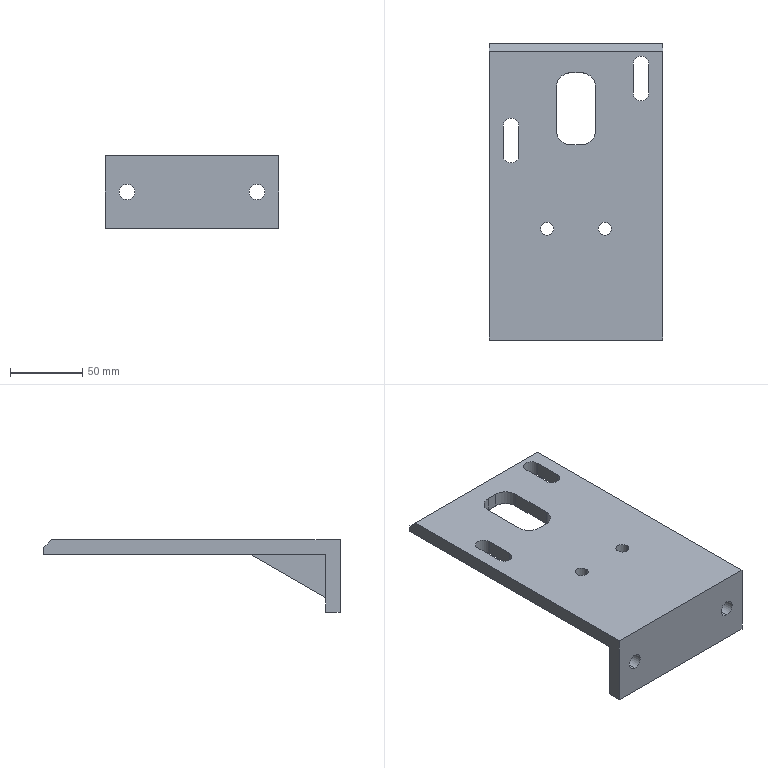NC program | NX | posted with a generic post | part box 120 x 205 x 50 mm
Lines 10894 to 11006 of 11006:
(PLANAR_MILL_COPY_COPY_COPY_COPY_COPY_COPY_1_COPY , TOOL : D6A45)
N21768 T01 M6
N21770 G54
N21772 G17 G0 G90 X-91.1 Y0.866 B0. C0. S9500 M3
N21774 G43 Z30. H1
N21776 Z0.5
N21778 G94 G1 Z-1. F1250.
N21780 G3 X-91.6 Y0. R1.
N21782 G1 Y-60.
N21784 G2 X-92.5 Y-60.9 R0.9
N21786 G1 X-102.5
N21788 G2 X-103.4 Y-60. R0.9
N21790 G1 Y60.
N21792 G2 X-102.5 Y60.9 R0.9
N21794 G1 X-92.5
N21796 G2 X-91.6 Y60. R0.9
N21798 G1 Y0.
N21800 G3 X-91.1 Y-0.866 R1.
N21802 G1 Z0.5
N21804 G0 Z30.
(PLANAR_MILL_COPY_COPY_COPY_COPY_COPY_COPY_1_COPY_COPY , TOOL : D6A45)
N21806 X-23.851 Y21.744
N21808 Z-39.5
N21810 G1 Z-41.
N21812 X-24.634 Y23.1
N21814 G3 X-25.5 Y23.6 R1.
N21816 X-29.1 Y20. R3.6
N21818 X-25.5 Y23.6 R-3.6
N21820 X-26.366 Y23.1 R1.
N21822 G1 X-27.149 Y21.744
N21824 Z-39.5
N21826 G0 Z30.
N21828 Y-21.744
N21830 Z-39.5
N21832 G1 Z-41.
N21834 X-26.366 Y-23.1
N21836 G3 X-25.5 Y-23.6 R1.
N21838 X-21.9 Y-20. R3.6
N21840 X-25.5 Y-23.6 R-3.6
N21842 X-24.634 Y-23.1 R1.
N21844 G1 X-23.851 Y-21.744
N21846 Z-39.5
N21848 G0 Z30.
N21850 X-88.408 Y62.313
N21852 Z-39.5
N21854 G1 Z-41.
N21856 X-88.857 Y61.865
N21858 G3 X-89.118 Y60.9 R1.
N21860 G1 X102.4
N21862 G2 X103.4 Y59.9 R1.
N21864 G1 Y-59.9
N21866 G2 X102.4 Y-60.9 R1.
N21868 G1 X-89.118
N21870 G3 X-88.857 Y-61.865 R1.
N21872 G1 X-88.408 Y-62.313
N21874 Z-39.5
N21876 G0 Z30.
N21878 X34.23 Y-48.4
N21880 Z-39.5
N21882 G1 Z-41.
N21884 X34.634 Y-49.1
N21886 G3 X35.5 Y-49.6 R1.
N21888 G1 X45.5
N21890 G3 X50.1 Y-45. R4.6
N21892 X45.5 Y-40.4 R4.6
N21894 G1 X25.5
N21896 G3 X20.9 Y-45. R4.6
N21898 X25.5 Y-49.6 R4.6
N21900 G1 X35.5
N21902 G3 X36.366 Y-49.1 R1.
N21904 G1 X36.77 Y-48.4
N21906 Z-39.5
N21908 G0 Z30.
N21910 X56.23 Y-11.4
N21912 Z-39.5
N21914 G1 Z-41.
N21916 X56.634 Y-12.1
N21918 G3 X57.5 Y-12.6 R1.
N21920 G1 X72.5
N21922 G3 X81.6 Y-3.5 R9.1
N21924 G1 Y3.5
N21926 G3 X72.5 Y12.6 R9.1
N21928 G1 X42.5
N21930 G3 X33.4 Y3.5 R9.1
N21932 G1 Y-3.5
N21934 G3 X42.5 Y-12.6 R9.1
N21936 G1 X57.5
N21938 G3 X58.366 Y-12.1 R1.
N21940 G1 X58.77 Y-11.4
N21942 Z-39.5
N21944 G0 Z30.
N21946 X79.77 Y48.4
N21948 Z-39.5
N21950 G1 Z-41.
N21952 X79.366 Y49.1
N21954 G3 X78.5 Y49.6 R1.
N21956 G1 X68.5
N21958 G3 X63.9 Y45. R4.6
N21960 X68.5 Y40.4 R4.6
N21962 G1 X88.5
N21964 G3 X93.1 Y45. R4.6
N21966 X88.5 Y49.6 R4.6
N21968 G1 X78.5
N21970 G3 X77.634 Y49.1 R1.
N21972 G1 X77.23 Y48.4
N21974 Z-39.5
N21976 G0 Z30.
N21978 M5
N21980 M2